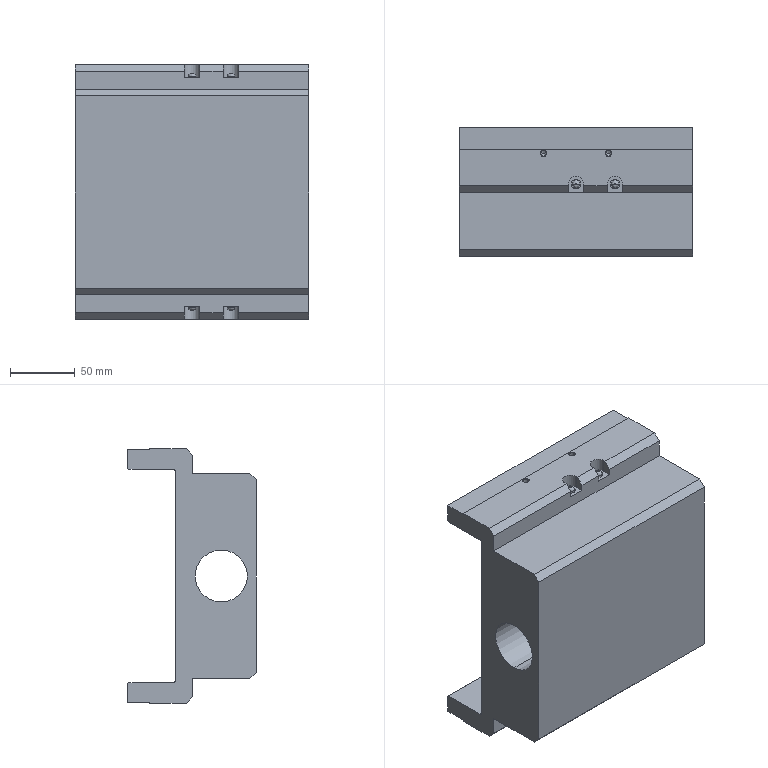Part | STEP file | ISPB-WXM-WA-750-10-200-T4-N-A1-AQ-B-EB^-Part-3 | 1 solid | 166 faces | box 180 x 99 x 196 mm | volume 1803389 mm3 | cylinder 68 | plane 58 | cone 32 | other 8 | commonest cylinder face diameters 8 x20 6.65 x16 4.134 x8 6 x8 7.5 x8 12 x4